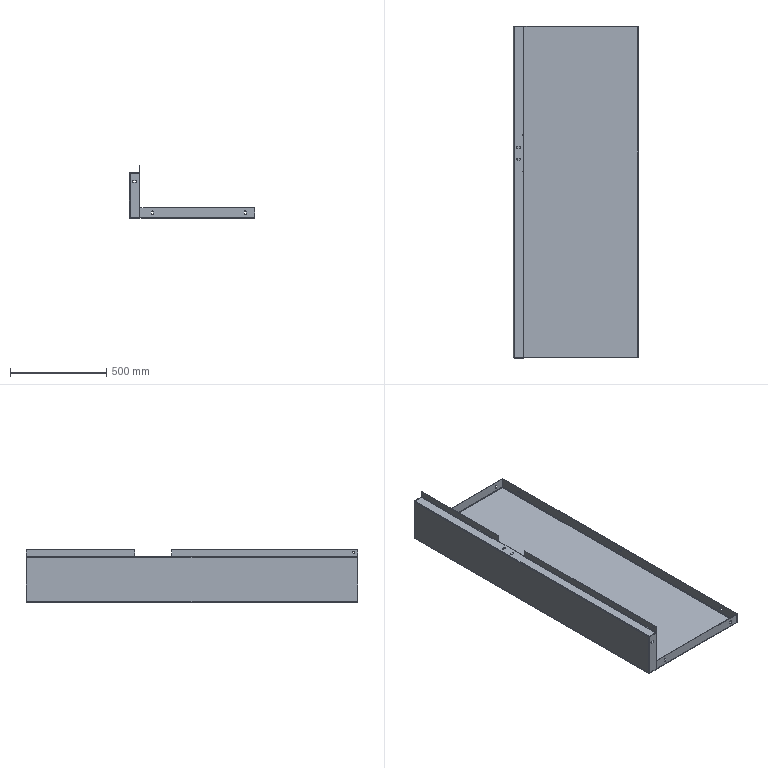Part | STEP file | SYL_0392D6J1SYL0380DJ100-382410 | 1 solid | 160 faces | box 650 x 1720 x 271 mm | volume 3661344 mm3 | plane 90 | cylinder 58 | spline 12 | commonest cylinder face diameters 10 x38 4 x9 8 x9 10.5 x2